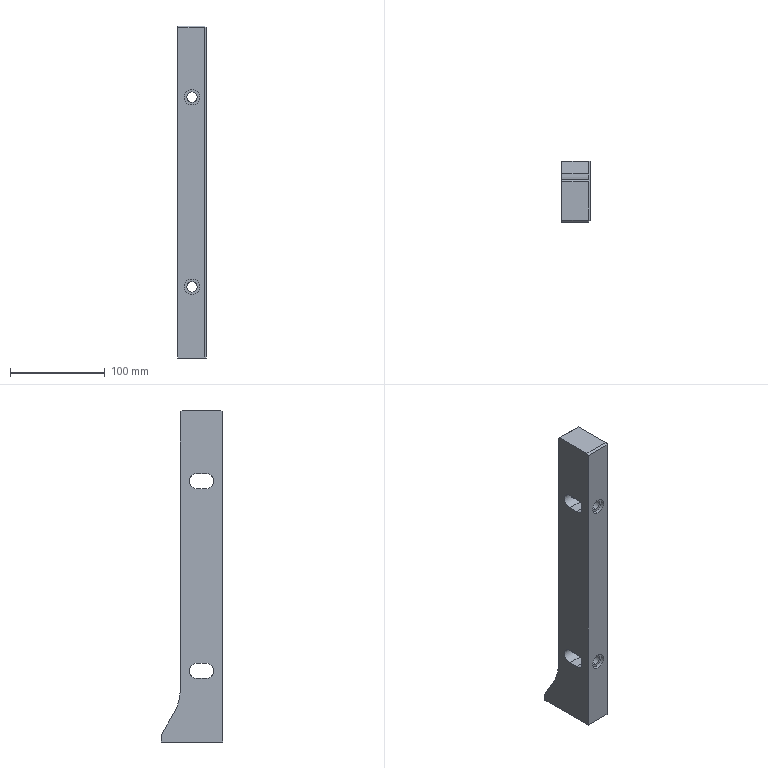Part | STEP file | Screen clamp fixing plate^Right screen clamp assembly_Screen assembly_PS-3045E-LDJ | 1 solid | 56 faces | box 30 x 64.5 x 350 mm | volume 453768 mm3 | cylinder 25 | plane 22 | cone 9 | commonest cylinder face diameters 5 x8 11 x8 16 x4 16.5 x4 100 x1